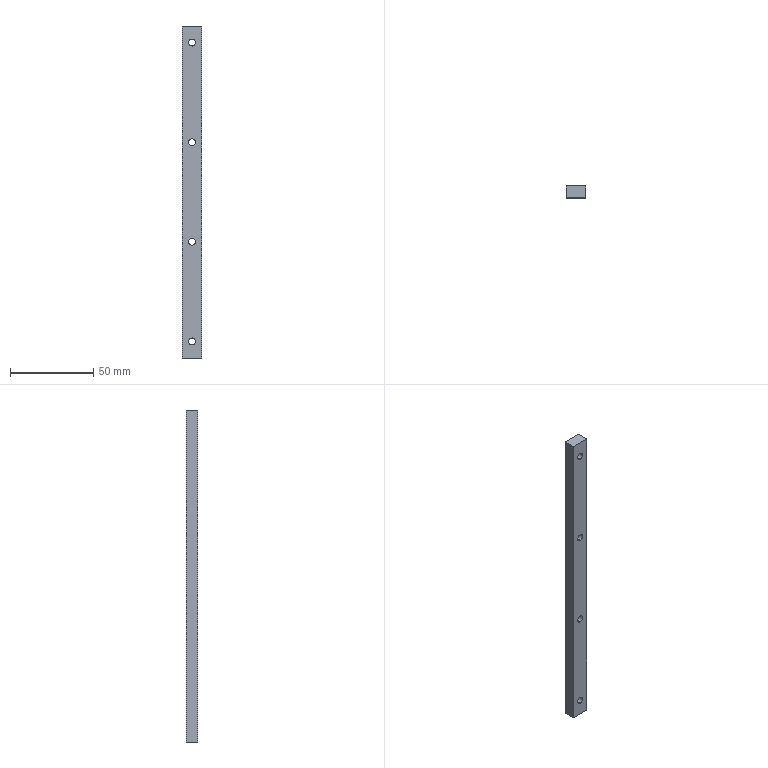Part | STEP file | Rãnh trượt | 1 solid | 14 faces | box 11.5 x 7 x 200 mm | volume 15712 mm3 | cylinder 8 | plane 6 | commonest cylinder face diameters 4.2 x8
STEP:
#1=CARTESIAN_POINT('',(0.,-3.5,-92.1));
#2=VERTEX_POINT('',#1);
#3=CARTESIAN_POINT('',(0.,-3.5,-87.9));
#4=VERTEX_POINT('',#3);
#5=CARTESIAN_POINT('',(0.,-3.5,-90.));
#6=DIRECTION('',(0.,1.,0.));
#7=DIRECTION('',(0.,0.,1.));
#8=AXIS2_PLACEMENT_3D('',#5,#6,#7);
#9=CIRCLE('',#8,2.1);
#10=EDGE_CURVE('',#2,#4,#9,.T.);
#11=ORIENTED_EDGE('',*,*,#10,.F.);
#12=CARTESIAN_POINT('',(0.,3.5,-92.1));
#13=VERTEX_POINT('',#12);
#14=CARTESIAN_POINT('',(0.,3.5,-92.1));
#15=DIRECTION('',(0.,1.,0.));
#16=VECTOR('',#15,1000.);
#17=LINE('',#14,#16);
#18=EDGE_CURVE('',#2,#13,#17,.T.);
#19=ORIENTED_EDGE('',*,*,#18,.T.);
#20=CARTESIAN_POINT('',(0.,3.5,-87.9));
#21=VERTEX_POINT('',#20);
#22=CARTESIAN_POINT('',(0.,3.5,-90.));
#23=DIRECTION('',(0.,1.,0.));
#24=DIRECTION('',(0.,0.,1.));
#25=AXIS2_PLACEMENT_3D('',#22,#23,#24);
#26=CIRCLE('',#25,2.1);
#27=EDGE_CURVE('',#13,#21,#26,.T.);
#28=ORIENTED_EDGE('',*,*,#27,.T.);
#29=CARTESIAN_POINT('',(0.,3.5,-87.9));
#30=DIRECTION('',(0.,1.,0.));
#31=VECTOR('',#30,1000.);
#32=LINE('',#29,#31);
#33=EDGE_CURVE('',#4,#21,#32,.T.);
#34=ORIENTED_EDGE('',*,*,#33,.F.);
#35=EDGE_LOOP('',(#11,#19,#28,#34));
#36=FACE_OUTER_BOUND('',#35,.T.);
#37=CARTESIAN_POINT('',(0.,3.5,-90.));
#38=DIRECTION('',(0.,1.,0.));
#39=DIRECTION('',(0.,0.,1.));
#40=AXIS2_PLACEMENT_3D('',#37,#38,#39);
#41=CYLINDRICAL_SURFACE('',#40,2.1);
#42=ADVANCED_FACE('',(#36),#41,.F.);
#43=CARTESIAN_POINT('',(0.,-3.5,-32.1));
#44=VERTEX_POINT('',#43);
#45=CARTESIAN_POINT('',(0.,-3.5,-27.9));
#46=VERTEX_POINT('',#45);
#47=CARTESIAN_POINT('',(0.,-3.5,-30.));
#48=DIRECTION('',(0.,1.,0.));
#49=DIRECTION('',(0.,0.,1.));
#50=AXIS2_PLACEMENT_3D('',#47,#48,#49);
#51=CIRCLE('',#50,2.1);
#52=EDGE_CURVE('',#44,#46,#51,.T.);
#53=ORIENTED_EDGE('',*,*,#52,.F.);
#54=CARTESIAN_POINT('',(0.,3.5,-32.1));
#55=VERTEX_POINT('',#54);
#56=CARTESIAN_POINT('',(0.,3.5,-32.1));
#57=DIRECTION('',(0.,1.,0.));
#58=VECTOR('',#57,1000.);
#59=LINE('',#56,#58);
#60=EDGE_CURVE('',#44,#55,#59,.T.);
#61=ORIENTED_EDGE('',*,*,#60,.T.);
#62=CARTESIAN_POINT('',(0.,3.5,-27.9));
#63=VERTEX_POINT('',#62);
#64=CARTESIAN_POINT('',(0.,3.5,-30.));
#65=DIRECTION('',(0.,1.,0.));
#66=DIRECTION('',(0.,0.,1.));
#67=AXIS2_PLACEMENT_3D('',#64,#65,#66);
#68=CIRCLE('',#67,2.1);
#69=EDGE_CURVE('',#55,#63,#68,.T.);
#70=ORIENTED_EDGE('',*,*,#69,.T.);
#71=CARTESIAN_POINT('',(0.,3.5,-27.9));
#72=DIRECTION('',(0.,1.,0.));
#73=VECTOR('',#72,1000.);
#74=LINE('',#71,#73);
#75=EDGE_CURVE('',#46,#63,#74,.T.);
#76=ORIENTED_EDGE('',*,*,#75,.F.);
#77=EDGE_LOOP('',(#53,#61,#70,#76));
#78=FACE_OUTER_BOUND('',#77,.T.);
#79=CARTESIAN_POINT('',(0.,3.5,-30.));
#80=DIRECTION('',(0.,1.,0.));
#81=DIRECTION('',(0.,0.,1.));
#82=AXIS2_PLACEMENT_3D('',#79,#80,#81);
#83=CYLINDRICAL_SURFACE('',#82,2.1);
#84=ADVANCED_FACE('',(#78),#83,.F.);
#85=CARTESIAN_POINT('',(0.,-3.5,27.9));
#86=VERTEX_POINT('',#85);
#87=CARTESIAN_POINT('',(0.,-3.5,32.1));
#88=VERTEX_POINT('',#87);
#89=CARTESIAN_POINT('',(0.,-3.5,30.));
#90=DIRECTION('',(0.,1.,0.));
#91=DIRECTION('',(0.,0.,1.));
#92=AXIS2_PLACEMENT_3D('',#89,#90,#91);
#93=CIRCLE('',#92,2.1);
#94=EDGE_CURVE('',#86,#88,#93,.T.);
#95=ORIENTED_EDGE('',*,*,#94,.F.);
#96=CARTESIAN_POINT('',(0.,3.5,27.9));
#97=VERTEX_POINT('',#96);
#98=CARTESIAN_POINT('',(0.,3.5,27.9));
#99=DIRECTION('',(0.,1.,0.));
#100=VECTOR('',#99,1000.);
#101=LINE('',#98,#100);
#102=EDGE_CURVE('',#86,#97,#101,.T.);
#103=ORIENTED_EDGE('',*,*,#102,.T.);
#104=CARTESIAN_POINT('',(0.,3.5,32.1));
#105=VERTEX_POINT('',#104);
#106=CARTESIAN_POINT('',(0.,3.5,30.));
#107=DIRECTION('',(0.,1.,0.));
#108=DIRECTION('',(0.,0.,1.));
#109=AXIS2_PLACEMENT_3D('',#106,#107,#108);
#110=CIRCLE('',#109,2.1);
#111=EDGE_CURVE('',#97,#105,#110,.T.);
#112=ORIENTED_EDGE('',*,*,#111,.T.);
#113=CARTESIAN_POINT('',(0.,3.5,32.1));
#114=DIRECTION('',(0.,1.,0.));
#115=VECTOR('',#114,1000.);
#116=LINE('',#113,#115);
#117=EDGE_CURVE('',#88,#105,#116,.T.);
#118=ORIENTED_EDGE('',*,*,#117,.F.);
#119=EDGE_LOOP('',(#95,#103,#112,#118));
#120=FACE_OUTER_BOUND('',#119,.T.);
#121=CARTESIAN_POINT('',(0.,3.5,30.));
#122=DIRECTION('',(0.,1.,0.));
#123=DIRECTION('',(0.,0.,1.));
#124=AXIS2_PLACEMENT_3D('',#121,#122,#123);
#125=CYLINDRICAL_SURFACE('',#124,2.1);
#126=ADVANCED_FACE('',(#120),#125,.F.);
#127=CARTESIAN_POINT('',(0.,-3.5,87.9));
#128=VERTEX_POINT('',#127);
#129=CARTESIAN_POINT('',(0.,-3.5,92.1));
#130=VERTEX_POINT('',#129);
#131=CARTESIAN_POINT('',(0.,-3.5,90.));
#132=DIRECTION('',(0.,1.,0.));
#133=DIRECTION('',(0.,0.,1.));
#134=AXIS2_PLACEMENT_3D('',#131,#132,#133);
#135=CIRCLE('',#134,2.1);
#136=EDGE_CURVE('',#128,#130,#135,.T.);
#137=ORIENTED_EDGE('',*,*,#136,.F.);
#138=CARTESIAN_POINT('',(0.,3.5,87.9));
#139=VERTEX_POINT('',#138);
#140=CARTESIAN_POINT('',(0.,3.5,87.9));
#141=DIRECTION('',(0.,1.,0.));
#142=VECTOR('',#141,1000.);
#143=LINE('',#140,#142);
#144=EDGE_CURVE('',#128,#139,#143,.T.);
#145=ORIENTED_EDGE('',*,*,#144,.T.);
#146=CARTESIAN_POINT('',(0.,3.5,92.1));
#147=VERTEX_POINT('',#146);
#148=CARTESIAN_POINT('',(0.,3.5,90.));
#149=DIRECTION('',(0.,1.,0.));
#150=DIRECTION('',(0.,0.,1.));
#151=AXIS2_PLACEMENT_3D('',#148,#149,#150);
#152=CIRCLE('',#151,2.1);
#153=EDGE_CURVE('',#139,#147,#152,.T.);
#154=ORIENTED_EDGE('',*,*,#153,.T.);
#155=CARTESIAN_POINT('',(0.,3.5,92.1));
#156=DIRECTION('',(0.,1.,0.));
#157=VECTOR('',#156,1000.);
#158=LINE('',#155,#157);
#159=EDGE_CURVE('',#130,#147,#158,.T.);
#160=ORIENTED_EDGE('',*,*,#159,.F.);
#161=EDGE_LOOP('',(#137,#145,#154,#160));
#162=FACE_OUTER_BOUND('',#161,.T.);
#163=CARTESIAN_POINT('',(0.,3.5,90.));
#164=DIRECTION('',(0.,1.,0.));
#165=DIRECTION('',(0.,0.,1.));
#166=AXIS2_PLACEMENT_3D('',#163,#164,#165);
#167=CYLINDRICAL_SURFACE('',#166,2.1);
#168=ADVANCED_FACE('',(#162),#167,.F.);
#169=CARTESIAN_POINT('',(5.75,-3.5,-100.));
#170=VERTEX_POINT('',#169);
#171=CARTESIAN_POINT('',(5.75,3.5,-100.));
#172=VERTEX_POINT('',#171);
#173=CARTESIAN_POINT('',(5.75,-3.5,-100.));
#174=DIRECTION('',(0.,1.,0.));
#175=VECTOR('',#174,1000.);
#176=LINE('',#173,#175);
#177=EDGE_CURVE('',#170,#172,#176,.T.);
#178=ORIENTED_EDGE('',*,*,#177,.T.);
#179=CARTESIAN_POINT('',(5.75,3.5,100.));
#180=VERTEX_POINT('',#179);
#181=CARTESIAN_POINT('',(5.75,3.5,100.));
#182=DIRECTION('',(0.,0.,-1.));
#183=VECTOR('',#182,1000.);
#184=LINE('',#181,#183);
#185=EDGE_CURVE('',#180,#172,#184,.T.);
#186=ORIENTED_EDGE('',*,*,#185,.F.);
#187=CARTESIAN_POINT('',(5.75,-3.5,100.));
#188=VERTEX_POINT('',#187);
#189=CARTESIAN_POINT('',(5.75,-3.5,100.));
#190=DIRECTION('',(0.,1.,0.));
#191=VECTOR('',#190,1000.);
#192=LINE('',#189,#191);
#193=EDGE_CURVE('',#188,#180,#192,.T.);
#194=ORIENTED_EDGE('',*,*,#193,.F.);
#195=CARTESIAN_POINT('',(5.75,-3.5,100.));
#196=DIRECTION('',(0.,0.,-1.));
#197=VECTOR('',#196,1000.);
#198=LINE('',#195,#197);
#199=EDGE_CURVE('',#188,#170,#198,.T.);
#200=ORIENTED_EDGE('',*,*,#199,.T.);
#201=EDGE_LOOP('',(#178,#186,#194,#200));
#202=FACE_OUTER_BOUND('',#201,.T.);
#203=CARTESIAN_POINT('',(5.75,-3.5,100.));
#204=DIRECTION('',(-1.,0.,0.));
#205=DIRECTION('',(0.,0.,1.));
#206=AXIS2_PLACEMENT_3D('',#203,#204,#205);
#207=PLANE('',#206);
#208=ADVANCED_FACE('',(#202),#207,.F.);
#209=CARTESIAN_POINT('',(0.,3.5,-90.));
#210=DIRECTION('',(0.,1.,0.));
#211=DIRECTION('',(0.,0.,1.));
#212=AXIS2_PLACEMENT_3D('',#209,#210,#211);
#213=CIRCLE('',#212,2.1);
#214=EDGE_CURVE('',#21,#13,#213,.T.);
#215=ORIENTED_EDGE('',*,*,#214,.F.);
#216=ORIENTED_EDGE('',*,*,#27,.F.);
#217=EDGE_LOOP('',(#215,#216));
#218=FACE_BOUND('',#217,.T.);
#219=CARTESIAN_POINT('',(0.,3.5,-30.));
#220=DIRECTION('',(0.,1.,0.));
#221=DIRECTION('',(0.,0.,1.));
#222=AXIS2_PLACEMENT_3D('',#219,#220,#221);
#223=CIRCLE('',#222,2.1);
#224=EDGE_CURVE('',#63,#55,#223,.T.);
#225=ORIENTED_EDGE('',*,*,#224,.F.);
#226=ORIENTED_EDGE('',*,*,#69,.F.);
#227=EDGE_LOOP('',(#225,#226));
#228=FACE_BOUND('',#227,.T.);
#229=CARTESIAN_POINT('',(0.,3.5,30.));
#230=DIRECTION('',(0.,1.,0.));
#231=DIRECTION('',(0.,0.,1.));
#232=AXIS2_PLACEMENT_3D('',#229,#230,#231);
#233=CIRCLE('',#232,2.1);
#234=EDGE_CURVE('',#105,#97,#233,.T.);
#235=ORIENTED_EDGE('',*,*,#234,.F.);
#236=ORIENTED_EDGE('',*,*,#111,.F.);
#237=EDGE_LOOP('',(#235,#236));
#238=FACE_BOUND('',#237,.T.);
#239=CARTESIAN_POINT('',(0.,3.5,90.));
#240=DIRECTION('',(0.,1.,0.));
#241=DIRECTION('',(0.,0.,1.));
#242=AXIS2_PLACEMENT_3D('',#239,#240,#241);
#243=CIRCLE('',#242,2.1);
#244=EDGE_CURVE('',#147,#139,#243,.T.);
#245=ORIENTED_EDGE('',*,*,#244,.F.);
#246=ORIENTED_EDGE('',*,*,#153,.F.);
#247=EDGE_LOOP('',(#245,#246));
#248=FACE_BOUND('',#247,.T.);
#249=CARTESIAN_POINT('',(-5.75,3.5,-100.));
#250=VERTEX_POINT('',#249);
#251=CARTESIAN_POINT('',(-5.75,3.5,-100.));
#252=DIRECTION('',(-1.,0.,0.));
#253=VECTOR('',#252,1000.);
#254=LINE('',#251,#253);
#255=EDGE_CURVE('',#172,#250,#254,.T.);
#256=ORIENTED_EDGE('',*,*,#255,.T.);
#257=CARTESIAN_POINT('',(-5.75,3.5,100.));
#258=VERTEX_POINT('',#257);
#259=CARTESIAN_POINT('',(-5.75,3.5,100.));
#260=DIRECTION('',(0.,0.,-1.));
#261=VECTOR('',#260,1000.);
#262=LINE('',#259,#261);
#263=EDGE_CURVE('',#258,#250,#262,.T.);
#264=ORIENTED_EDGE('',*,*,#263,.F.);
#265=CARTESIAN_POINT('',(-5.75,3.5,100.));
#266=DIRECTION('',(-1.,0.,0.));
#267=VECTOR('',#266,1000.);
#268=LINE('',#265,#267);
#269=EDGE_CURVE('',#180,#258,#268,.T.);
#270=ORIENTED_EDGE('',*,*,#269,.F.);
#271=ORIENTED_EDGE('',*,*,#185,.T.);
#272=EDGE_LOOP('',(#256,#264,#270,#271));
#273=FACE_OUTER_BOUND('',#272,.T.);
#274=CARTESIAN_POINT('',(-5.75,3.5,100.));
#275=DIRECTION('',(0.,-1.,0.));
#276=DIRECTION('',(0.,0.,-1.));
#277=AXIS2_PLACEMENT_3D('',#274,#275,#276);
#278=PLANE('',#277);
#279=ADVANCED_FACE('',(#218,#228,#238,#248,#273),#278,.F.);
#280=CARTESIAN_POINT('',(-5.75,-3.5,-100.));
#281=VERTEX_POINT('',#280);
#282=CARTESIAN_POINT('',(-5.75,-3.5,-100.));
#283=DIRECTION('',(0.,-1.,0.));
#284=VECTOR('',#283,1000.);
#285=LINE('',#282,#284);
#286=EDGE_CURVE('',#250,#281,#285,.T.);
#287=ORIENTED_EDGE('',*,*,#286,.T.);
#288=CARTESIAN_POINT('',(-5.75,-3.5,100.));
#289=VERTEX_POINT('',#288);
#290=CARTESIAN_POINT('',(-5.75,-3.5,100.));
#291=DIRECTION('',(0.,0.,-1.));
#292=VECTOR('',#291,1000.);
#293=LINE('',#290,#292);
#294=EDGE_CURVE('',#289,#281,#293,.T.);
#295=ORIENTED_EDGE('',*,*,#294,.F.);
#296=CARTESIAN_POINT('',(-5.75,-3.5,100.));
#297=DIRECTION('',(0.,-1.,0.));
#298=VECTOR('',#297,1000.);
#299=LINE('',#296,#298);
#300=EDGE_CURVE('',#258,#289,#299,.T.);
#301=ORIENTED_EDGE('',*,*,#300,.F.);
#302=ORIENTED_EDGE('',*,*,#263,.T.);
#303=EDGE_LOOP('',(#287,#295,#301,#302));
#304=FACE_OUTER_BOUND('',#303,.T.);
#305=CARTESIAN_POINT('',(-5.75,-3.5,100.));
#306=DIRECTION('',(1.,0.,0.));
#307=DIRECTION('',(0.,0.,-1.));
#308=AXIS2_PLACEMENT_3D('',#305,#306,#307);
#309=PLANE('',#308);
#310=ADVANCED_FACE('',(#304),#309,.F.);
#311=CARTESIAN_POINT('',(0.,-3.5,-90.));
#312=DIRECTION('',(0.,1.,0.));
#313=DIRECTION('',(0.,0.,1.));
#314=AXIS2_PLACEMENT_3D('',#311,#312,#313);
#315=CIRCLE('',#314,2.1);
#316=EDGE_CURVE('',#4,#2,#315,.T.);
#317=ORIENTED_EDGE('',*,*,#316,.T.);
#318=ORIENTED_EDGE('',*,*,#10,.T.);
#319=EDGE_LOOP('',(#317,#318));
#320=FACE_BOUND('',#319,.T.);
#321=CARTESIAN_POINT('',(0.,-3.5,-30.));
#322=DIRECTION('',(0.,1.,0.));
#323=DIRECTION('',(0.,0.,1.));
#324=AXIS2_PLACEMENT_3D('',#321,#322,#323);
#325=CIRCLE('',#324,2.1);
#326=EDGE_CURVE('',#46,#44,#325,.T.);
#327=ORIENTED_EDGE('',*,*,#326,.T.);
#328=ORIENTED_EDGE('',*,*,#52,.T.);
#329=EDGE_LOOP('',(#327,#328));
#330=FACE_BOUND('',#329,.T.);
#331=CARTESIAN_POINT('',(0.,-3.5,30.));
#332=DIRECTION('',(0.,1.,0.));
#333=DIRECTION('',(0.,0.,1.));
#334=AXIS2_PLACEMENT_3D('',#331,#332,#333);
#335=CIRCLE('',#334,2.1);
#336=EDGE_CURVE('',#88,#86,#335,.T.);
#337=ORIENTED_EDGE('',*,*,#336,.T.);
#338=ORIENTED_EDGE('',*,*,#94,.T.);
#339=EDGE_LOOP('',(#337,#338));
#340=FACE_BOUND('',#339,.T.);
#341=CARTESIAN_POINT('',(0.,-3.5,90.));
#342=DIRECTION('',(0.,1.,0.));
#343=DIRECTION('',(0.,0.,1.));
#344=AXIS2_PLACEMENT_3D('',#341,#342,#343);
#345=CIRCLE('',#344,2.1);
#346=EDGE_CURVE('',#130,#128,#345,.T.);
#347=ORIENTED_EDGE('',*,*,#346,.T.);
#348=ORIENTED_EDGE('',*,*,#136,.T.);
#349=EDGE_LOOP('',(#347,#348));
#350=FACE_BOUND('',#349,.T.);
#351=CARTESIAN_POINT('',(-5.75,-3.5,-100.));
#352=DIRECTION('',(1.,0.,0.));
#353=VECTOR('',#352,1000.);
#354=LINE('',#351,#353);
#355=EDGE_CURVE('',#281,#170,#354,.T.);
#356=ORIENTED_EDGE('',*,*,#355,.T.);
#357=ORIENTED_EDGE('',*,*,#199,.F.);
#358=CARTESIAN_POINT('',(-5.75,-3.5,100.));
#359=DIRECTION('',(1.,0.,0.));
#360=VECTOR('',#359,1000.);
#361=LINE('',#358,#360);
#362=EDGE_CURVE('',#289,#188,#361,.T.);
#363=ORIENTED_EDGE('',*,*,#362,.F.);
#364=ORIENTED_EDGE('',*,*,#294,.T.);
#365=EDGE_LOOP('',(#356,#357,#363,#364));
#366=FACE_OUTER_BOUND('',#365,.T.);
#367=CARTESIAN_POINT('',(-5.75,-3.5,100.));
#368=DIRECTION('',(0.,1.,0.));
#369=DIRECTION('',(0.,0.,1.));
#370=AXIS2_PLACEMENT_3D('',#367,#368,#369);
#371=PLANE('',#370);
#372=ADVANCED_FACE('',(#320,#330,#340,#350,#366),#371,.F.);
#373=ORIENTED_EDGE('',*,*,#193,.T.);
#374=ORIENTED_EDGE('',*,*,#269,.T.);
#375=ORIENTED_EDGE('',*,*,#300,.T.);
#376=ORIENTED_EDGE('',*,*,#362,.T.);
#377=EDGE_LOOP('',(#373,#374,#375,#376));
#378=FACE_OUTER_BOUND('',#377,.T.);
#379=CARTESIAN_POINT('',(0.,0.,100.));
#380=DIRECTION('',(0.,0.,-1.));
#381=DIRECTION('',(-1.,0.,0.));
#382=AXIS2_PLACEMENT_3D('',#379,#380,#381);
#383=PLANE('',#382);
#384=ADVANCED_FACE('',(#378),#383,.F.);
#385=ORIENTED_EDGE('',*,*,#177,.F.);
#386=ORIENTED_EDGE('',*,*,#355,.F.);
#387=ORIENTED_EDGE('',*,*,#286,.F.);
#388=ORIENTED_EDGE('',*,*,#255,.F.);
#389=EDGE_LOOP('',(#385,#386,#387,#388));
#390=FACE_OUTER_BOUND('',#389,.T.);
#391=CARTESIAN_POINT('',(0.,0.,-100.));
#392=DIRECTION('',(0.,0.,-1.));
#393=DIRECTION('',(-1.,0.,0.));
#394=AXIS2_PLACEMENT_3D('',#391,#392,#393);
#395=PLANE('',#394);
#396=ADVANCED_FACE('',(#390),#395,.T.);
#397=ORIENTED_EDGE('',*,*,#144,.F.);
#398=ORIENTED_EDGE('',*,*,#346,.F.);
#399=ORIENTED_EDGE('',*,*,#159,.T.);
#400=ORIENTED_EDGE('',*,*,#244,.T.);
#401=EDGE_LOOP('',(#397,#398,#399,#400));
#402=FACE_OUTER_BOUND('',#401,.T.);
#403=CARTESIAN_POINT('',(0.,3.5,90.));
#404=DIRECTION('',(0.,1.,0.));
#405=DIRECTION('',(0.,0.,1.));
#406=AXIS2_PLACEMENT_3D('',#403,#404,#405);
#407=CYLINDRICAL_SURFACE('',#406,2.1);
#408=ADVANCED_FACE('',(#402),#407,.F.);
#409=ORIENTED_EDGE('',*,*,#102,.F.);
#410=ORIENTED_EDGE('',*,*,#336,.F.);
#411=ORIENTED_EDGE('',*,*,#117,.T.);
#412=ORIENTED_EDGE('',*,*,#234,.T.);
#413=EDGE_LOOP('',(#409,#410,#411,#412));
#414=FACE_OUTER_BOUND('',#413,.T.);
#415=CARTESIAN_POINT('',(0.,3.5,30.));
#416=DIRECTION('',(0.,1.,0.));
#417=DIRECTION('',(0.,0.,1.));
#418=AXIS2_PLACEMENT_3D('',#415,#416,#417);
#419=CYLINDRICAL_SURFACE('',#418,2.1);
#420=ADVANCED_FACE('',(#414),#419,.F.);
#421=ORIENTED_EDGE('',*,*,#60,.F.);
#422=ORIENTED_EDGE('',*,*,#326,.F.);
#423=ORIENTED_EDGE('',*,*,#75,.T.);
#424=ORIENTED_EDGE('',*,*,#224,.T.);
#425=EDGE_LOOP('',(#421,#422,#423,#424));
#426=FACE_OUTER_BOUND('',#425,.T.);
#427=CARTESIAN_POINT('',(0.,3.5,-30.));
#428=DIRECTION('',(0.,1.,0.));
#429=DIRECTION('',(0.,0.,1.));
#430=AXIS2_PLACEMENT_3D('',#427,#428,#429);
#431=CYLINDRICAL_SURFACE('',#430,2.1);
#432=ADVANCED_FACE('',(#426),#431,.F.);
#433=ORIENTED_EDGE('',*,*,#18,.F.);
#434=ORIENTED_EDGE('',*,*,#316,.F.);
#435=ORIENTED_EDGE('',*,*,#33,.T.);
#436=ORIENTED_EDGE('',*,*,#214,.T.);
#437=EDGE_LOOP('',(#433,#434,#435,#436));
#438=FACE_OUTER_BOUND('',#437,.T.);
#439=CARTESIAN_POINT('',(0.,3.5,-90.));
#440=DIRECTION('',(0.,1.,0.));
#441=DIRECTION('',(0.,0.,1.));
#442=AXIS2_PLACEMENT_3D('',#439,#440,#441);
#443=CYLINDRICAL_SURFACE('',#442,2.1);
#444=ADVANCED_FACE('',(#438),#443,.F.);
#445=CLOSED_SHELL('',(#42,#84,#126,#168,#208,#279,#310,#372,#384,#396,#408,#420,#432,#444));
#446=MANIFOLD_SOLID_BREP('',#445);
#447=CARTESIAN_POINT('',(0.,0.,0.));
#448=DIRECTION('',(0.,0.,1.));
#449=DIRECTION('',(1.,0.,0.));
#450=AXIS2_PLACEMENT_3D('',#447,#448,#449);
#451=(LENGTH_UNIT()NAMED_UNIT(*)SI_UNIT(.MILLI.,.METRE.));
#452=UNCERTAINTY_MEASURE_WITH_UNIT(LENGTH_MEASURE(0.00001),#451,'','');
#453=(NAMED_UNIT(*)PLANE_ANGLE_UNIT()SI_UNIT($,.RADIAN.));
#454=(NAMED_UNIT(*)SI_UNIT($,.STERADIAN.)SOLID_ANGLE_UNIT());
#455=(GEOMETRIC_REPRESENTATION_CONTEXT(3)GLOBAL_UNCERTAINTY_ASSIGNED_CONTEXT((#452))GLOBAL_UNIT_ASSIGNED_CONTEXT((#451,#453,#454))REPRESENTATION_CONTEXT('',''));
#456=ADVANCED_BREP_SHAPE_REPRESENTATION('',(#446,#450),#455);